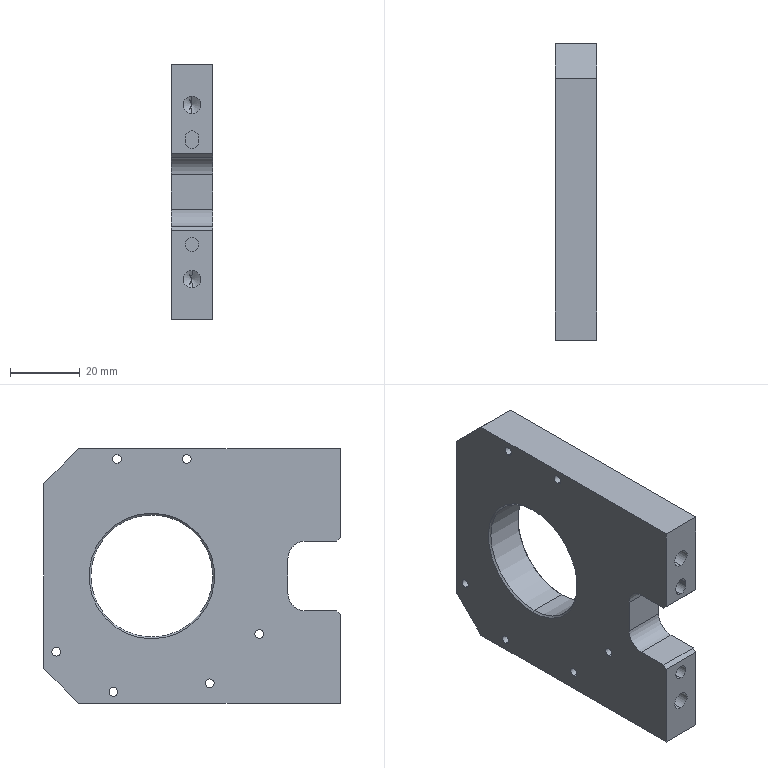Part | SolidWorks | features Chamfer 3, HoleWzd 2, Extrusion 1, ICE 1 | 1 solid | 51 faces | box 12 x 85 x 73 mm | volume 56726 mm3 | cylinder 25 | plane 18 | cone 8 | commonest cylinder face diameters 2.5 x12 4 x5 5 x4 10 x2 35 x2
STEP:
#1=CARTESIAN_POINT('',(5.5,54.,17.5));
#2=VERTEX_POINT('',#1);
#3=CARTESIAN_POINT('',(5.5,54.,-17.5));
#4=VERTEX_POINT('',#3);
#5=CARTESIAN_POINT('',(5.5,54.,0.));
#6=DIRECTION('',(1.,0.,0.));
#7=DIRECTION('',(0.,0.,1.));
#8=AXIS2_PLACEMENT_3D('',#5,#6,#7);
#9=CIRCLE('',#8,17.5);
#10=EDGE_CURVE('',#2,#4,#9,.T.);
#11=ORIENTED_EDGE('',*,*,#10,.F.);
#12=CARTESIAN_POINT('',(6.,54.,18.));
#13=VERTEX_POINT('',#12);
#14=CARTESIAN_POINT('',(5.5,54.,17.5));
#15=DIRECTION('',(0.7071,0.,0.7071));
#16=VECTOR('',#15,1000.);
#17=LINE('',#14,#16);
#18=EDGE_CURVE('',#2,#13,#17,.T.);
#19=ORIENTED_EDGE('',*,*,#18,.T.);
#20=CARTESIAN_POINT('',(6.,54.,-18.));
#21=VERTEX_POINT('',#20);
#22=CARTESIAN_POINT('',(6.,54.,0.));
#23=DIRECTION('',(-1.,0.,0.));
#24=DIRECTION('',(0.,0.,1.));
#25=AXIS2_PLACEMENT_3D('',#22,#23,#24);
#26=CIRCLE('',#25,18.);
#27=EDGE_CURVE('',#21,#13,#26,.T.);
#28=ORIENTED_EDGE('',*,*,#27,.F.);
#29=CARTESIAN_POINT('',(5.5,54.,-17.5));
#30=DIRECTION('',(0.7071,0.,-0.7071));
#31=VECTOR('',#30,1000.);
#32=LINE('',#29,#31);
#33=EDGE_CURVE('',#4,#21,#32,.T.);
#34=ORIENTED_EDGE('',*,*,#33,.F.);
#35=EDGE_LOOP('',(#11,#19,#28,#34));
#36=FACE_OUTER_BOUND('',#35,.T.);
#37=CARTESIAN_POINT('',(5.5,54.,0.));
#38=DIRECTION('',(1.,0.,0.));
#39=DIRECTION('',(0.,0.,-1.));
#40=AXIS2_PLACEMENT_3D('',#37,#38,#39);
#41=CONICAL_SURFACE('',#40,17.5,0.7854);
#42=ADVANCED_FACE('',(#36),#41,.F.);
#43=CARTESIAN_POINT('',(-5.5,54.,-17.5));
#44=VERTEX_POINT('',#43);
#45=CARTESIAN_POINT('',(-5.5,54.,17.5));
#46=VERTEX_POINT('',#45);
#47=CARTESIAN_POINT('',(-5.5,54.,0.));
#48=DIRECTION('',(-1.,0.,0.));
#49=DIRECTION('',(0.,0.,1.));
#50=AXIS2_PLACEMENT_3D('',#47,#48,#49);
#51=CIRCLE('',#50,17.5);
#52=EDGE_CURVE('',#44,#46,#51,.T.);
#53=ORIENTED_EDGE('',*,*,#52,.F.);
#54=CARTESIAN_POINT('',(-6.,54.,-18.));
#55=VERTEX_POINT('',#54);
#56=CARTESIAN_POINT('',(-6.,54.,-18.));
#57=DIRECTION('',(-0.7071,0.,-0.7071));
#58=VECTOR('',#57,1000.);
#59=LINE('',#56,#58);
#60=EDGE_CURVE('',#44,#55,#59,.T.);
#61=ORIENTED_EDGE('',*,*,#60,.T.);
#62=CARTESIAN_POINT('',(-6.,54.,18.));
#63=VERTEX_POINT('',#62);
#64=CARTESIAN_POINT('',(-6.,54.,0.));
#65=DIRECTION('',(1.,0.,0.));
#66=DIRECTION('',(0.,0.,1.));
#67=AXIS2_PLACEMENT_3D('',#64,#65,#66);
#68=CIRCLE('',#67,18.);
#69=EDGE_CURVE('',#63,#55,#68,.T.);
#70=ORIENTED_EDGE('',*,*,#69,.F.);
#71=CARTESIAN_POINT('',(-6.,54.,18.));
#72=DIRECTION('',(-0.7071,0.,0.7071));
#73=VECTOR('',#72,1000.);
#74=LINE('',#71,#73);
#75=EDGE_CURVE('',#46,#63,#74,.T.);
#76=ORIENTED_EDGE('',*,*,#75,.F.);
#77=EDGE_LOOP('',(#53,#61,#70,#76));
#78=FACE_OUTER_BOUND('',#77,.T.);
#79=CARTESIAN_POINT('',(-6.,54.,0.));
#80=DIRECTION('',(-1.,0.,0.));
#81=DIRECTION('',(0.,0.,1.));
#82=AXIS2_PLACEMENT_3D('',#79,#80,#81);
#83=CONICAL_SURFACE('',#82,18.,0.7854);
#84=ADVANCED_FACE('',(#78),#83,.F.);
#85=CARTESIAN_POINT('',(6.,44.,32.25));
#86=VERTEX_POINT('',#85);
#87=CARTESIAN_POINT('',(6.,44.,34.75));
#88=VERTEX_POINT('',#87);
#89=CARTESIAN_POINT('',(6.,44.,33.5));
#90=DIRECTION('',(-1.,0.,0.));
#91=DIRECTION('',(0.,0.,1.));
#92=AXIS2_PLACEMENT_3D('',#89,#90,#91);
#93=CIRCLE('',#92,1.25);
#94=EDGE_CURVE('',#86,#88,#93,.T.);
#95=ORIENTED_EDGE('',*,*,#94,.F.);
#96=CARTESIAN_POINT('',(-6.,44.,32.25));
#97=VERTEX_POINT('',#96);
#98=CARTESIAN_POINT('',(-6.,44.,32.25));
#99=DIRECTION('',(-1.,0.,0.));
#100=VECTOR('',#99,1000.);
#101=LINE('',#98,#100);
#102=EDGE_CURVE('',#86,#97,#101,.T.);
#103=ORIENTED_EDGE('',*,*,#102,.T.);
#104=CARTESIAN_POINT('',(-6.,44.,34.75));
#105=VERTEX_POINT('',#104);
#106=CARTESIAN_POINT('',(-6.,44.,33.5));
#107=DIRECTION('',(-1.,0.,0.));
#108=DIRECTION('',(0.,0.,1.));
#109=AXIS2_PLACEMENT_3D('',#106,#107,#108);
#110=CIRCLE('',#109,1.25);
#111=EDGE_CURVE('',#97,#105,#110,.T.);
#112=ORIENTED_EDGE('',*,*,#111,.T.);
#113=CARTESIAN_POINT('',(-6.,44.,34.75));
#114=DIRECTION('',(-1.,0.,0.));
#115=VECTOR('',#114,1000.);
#116=LINE('',#113,#115);
#117=EDGE_CURVE('',#88,#105,#116,.T.);
#118=ORIENTED_EDGE('',*,*,#117,.F.);
#119=EDGE_LOOP('',(#95,#103,#112,#118));
#120=FACE_OUTER_BOUND('',#119,.T.);
#121=CARTESIAN_POINT('',(-6.,44.,33.5));
#122=DIRECTION('',(-1.,0.,0.));
#123=DIRECTION('',(0.,0.,1.));
#124=AXIS2_PLACEMENT_3D('',#121,#122,#123);
#125=CYLINDRICAL_SURFACE('',#124,1.25);
#126=ADVANCED_FACE('',(#120),#125,.F.);
#127=CARTESIAN_POINT('',(6.,64.,32.25));
#128=VERTEX_POINT('',#127);
#129=CARTESIAN_POINT('',(6.,64.,34.75));
#130=VERTEX_POINT('',#129);
#131=CARTESIAN_POINT('',(6.,64.,33.5));
#132=DIRECTION('',(-1.,0.,0.));
#133=DIRECTION('',(0.,0.,1.));
#134=AXIS2_PLACEMENT_3D('',#131,#132,#133);
#135=CIRCLE('',#134,1.25);
#136=EDGE_CURVE('',#128,#130,#135,.T.);
#137=ORIENTED_EDGE('',*,*,#136,.F.);
#138=CARTESIAN_POINT('',(-6.,64.,32.25));
#139=VERTEX_POINT('',#138);
#140=CARTESIAN_POINT('',(-6.,64.,32.25));
#141=DIRECTION('',(-1.,0.,0.));
#142=VECTOR('',#141,1000.);
#143=LINE('',#140,#142);
#144=EDGE_CURVE('',#128,#139,#143,.T.);
#145=ORIENTED_EDGE('',*,*,#144,.T.);
#146=CARTESIAN_POINT('',(-6.,64.,34.75));
#147=VERTEX_POINT('',#146);
#148=CARTESIAN_POINT('',(-6.,64.,33.5));
#149=DIRECTION('',(-1.,0.,0.));
#150=DIRECTION('',(0.,0.,1.));
#151=AXIS2_PLACEMENT_3D('',#148,#149,#150);
#152=CIRCLE('',#151,1.25);
#153=EDGE_CURVE('',#139,#147,#152,.T.);
#154=ORIENTED_EDGE('',*,*,#153,.T.);
#155=CARTESIAN_POINT('',(-6.,64.,34.75));
#156=DIRECTION('',(-1.,0.,0.));
#157=VECTOR('',#156,1000.);
#158=LINE('',#155,#157);
#159=EDGE_CURVE('',#130,#147,#158,.T.);
#160=ORIENTED_EDGE('',*,*,#159,.F.);
#161=EDGE_LOOP('',(#137,#145,#154,#160));
#162=FACE_OUTER_BOUND('',#161,.T.);
#163=CARTESIAN_POINT('',(-6.,64.,33.5));
#164=DIRECTION('',(-1.,0.,0.));
#165=DIRECTION('',(0.,0.,1.));
#166=AXIS2_PLACEMENT_3D('',#163,#164,#165);
#167=CYLINDRICAL_SURFACE('',#166,1.25);
#168=ADVANCED_FACE('',(#162),#167,.F.);
#169=CARTESIAN_POINT('',(6.,23.241,-17.867));
#170=VERTEX_POINT('',#169);
#171=CARTESIAN_POINT('',(6.,23.241,-15.367));
#172=VERTEX_POINT('',#171);
#173=CARTESIAN_POINT('',(6.,23.241,-16.617));
#174=DIRECTION('',(-1.,0.,0.));
#175=DIRECTION('',(0.,0.,1.));
#176=AXIS2_PLACEMENT_3D('',#173,#174,#175);
#177=CIRCLE('',#176,1.25);
#178=EDGE_CURVE('',#170,#172,#177,.T.);
#179=ORIENTED_EDGE('',*,*,#178,.F.);
#180=CARTESIAN_POINT('',(-6.,23.241,-17.867));
#181=VERTEX_POINT('',#180);
#182=CARTESIAN_POINT('',(-6.,23.241,-17.867));
#183=DIRECTION('',(-1.,0.,0.));
#184=VECTOR('',#183,1000.);
#185=LINE('',#182,#184);
#186=EDGE_CURVE('',#170,#181,#185,.T.);
#187=ORIENTED_EDGE('',*,*,#186,.T.);
#188=CARTESIAN_POINT('',(-6.,23.241,-15.367));
#189=VERTEX_POINT('',#188);
#190=CARTESIAN_POINT('',(-6.,23.241,-16.617));
#191=DIRECTION('',(-1.,0.,0.));
#192=DIRECTION('',(0.,0.,1.));
#193=AXIS2_PLACEMENT_3D('',#190,#191,#192);
#194=CIRCLE('',#193,1.25);
#195=EDGE_CURVE('',#181,#189,#194,.T.);
#196=ORIENTED_EDGE('',*,*,#195,.T.);
#197=CARTESIAN_POINT('',(-6.,23.241,-15.367));
#198=DIRECTION('',(-1.,0.,0.));
#199=VECTOR('',#198,1000.);
#200=LINE('',#197,#199);
#201=EDGE_CURVE('',#172,#189,#200,.T.);
#202=ORIENTED_EDGE('',*,*,#201,.F.);
#203=EDGE_LOOP('',(#179,#187,#196,#202));
#204=FACE_OUTER_BOUND('',#203,.T.);
#205=CARTESIAN_POINT('',(-6.,23.241,-16.617));
#206=DIRECTION('',(-1.,0.,0.));
#207=DIRECTION('',(0.,0.,1.));
#208=AXIS2_PLACEMENT_3D('',#205,#206,#207);
#209=CYLINDRICAL_SURFACE('',#208,1.25);
#210=ADVANCED_FACE('',(#204),#209,.F.);
#211=CARTESIAN_POINT('',(6.,37.383,-32.009));
#212=VERTEX_POINT('',#211);
#213=CARTESIAN_POINT('',(6.,37.383,-29.509));
#214=VERTEX_POINT('',#213);
#215=CARTESIAN_POINT('',(6.,37.383,-30.759));
#216=DIRECTION('',(-1.,0.,0.));
#217=DIRECTION('',(0.,0.,1.));
#218=AXIS2_PLACEMENT_3D('',#215,#216,#217);
#219=CIRCLE('',#218,1.25);
#220=EDGE_CURVE('',#212,#214,#219,.T.);
#221=ORIENTED_EDGE('',*,*,#220,.F.);
#222=CARTESIAN_POINT('',(-6.,37.383,-32.009));
#223=VERTEX_POINT('',#222);
#224=CARTESIAN_POINT('',(-6.,37.383,-32.009));
#225=DIRECTION('',(-1.,0.,0.));
#226=VECTOR('',#225,1000.);
#227=LINE('',#224,#226);
#228=EDGE_CURVE('',#212,#223,#227,.T.);
#229=ORIENTED_EDGE('',*,*,#228,.T.);
#230=CARTESIAN_POINT('',(-6.,37.383,-29.509));
#231=VERTEX_POINT('',#230);
#232=CARTESIAN_POINT('',(-6.,37.383,-30.759));
#233=DIRECTION('',(-1.,0.,0.));
#234=DIRECTION('',(0.,0.,1.));
#235=AXIS2_PLACEMENT_3D('',#232,#233,#234);
#236=CIRCLE('',#235,1.25);
#237=EDGE_CURVE('',#223,#231,#236,.T.);
#238=ORIENTED_EDGE('',*,*,#237,.T.);
#239=CARTESIAN_POINT('',(-6.,37.383,-29.509));
#240=DIRECTION('',(-1.,0.,0.));
#241=VECTOR('',#240,1000.);
#242=LINE('',#239,#241);
#243=EDGE_CURVE('',#214,#231,#242,.T.);
#244=ORIENTED_EDGE('',*,*,#243,.F.);
#245=EDGE_LOOP('',(#221,#229,#238,#244));
#246=FACE_OUTER_BOUND('',#245,.T.);
#247=CARTESIAN_POINT('',(-6.,37.383,-30.759));
#248=DIRECTION('',(-1.,0.,0.));
#249=DIRECTION('',(0.,0.,1.));
#250=AXIS2_PLACEMENT_3D('',#247,#248,#249);
#251=CYLINDRICAL_SURFACE('',#250,1.25);
#252=ADVANCED_FACE('',(#246),#251,.F.);
#253=CARTESIAN_POINT('',(6.,65.023,-34.427));
#254=VERTEX_POINT('',#253);
#255=CARTESIAN_POINT('',(6.,65.023,-31.927));
#256=VERTEX_POINT('',#255);
#257=CARTESIAN_POINT('',(6.,65.023,-33.177));
#258=DIRECTION('',(-1.,0.,0.));
#259=DIRECTION('',(0.,0.,1.));
#260=AXIS2_PLACEMENT_3D('',#257,#258,#259);
#261=CIRCLE('',#260,1.25);
#262=EDGE_CURVE('',#254,#256,#261,.T.);
#263=ORIENTED_EDGE('',*,*,#262,.F.);
#264=CARTESIAN_POINT('',(-6.,65.023,-34.427));
#265=VERTEX_POINT('',#264);
#266=CARTESIAN_POINT('',(-6.,65.023,-34.427));
#267=DIRECTION('',(-1.,0.,0.));
#268=VECTOR('',#267,1000.);
#269=LINE('',#266,#268);
#270=EDGE_CURVE('',#254,#265,#269,.T.);
#271=ORIENTED_EDGE('',*,*,#270,.T.);
#272=CARTESIAN_POINT('',(-6.,65.023,-31.927));
#273=VERTEX_POINT('',#272);
#274=CARTESIAN_POINT('',(-6.,65.023,-33.177));
#275=DIRECTION('',(-1.,0.,0.));
#276=DIRECTION('',(0.,0.,1.));
#277=AXIS2_PLACEMENT_3D('',#274,#275,#276);
#278=CIRCLE('',#277,1.25);
#279=EDGE_CURVE('',#265,#273,#278,.T.);
#280=ORIENTED_EDGE('',*,*,#279,.T.);
#281=CARTESIAN_POINT('',(-6.,65.023,-31.927));
#282=DIRECTION('',(-1.,0.,0.));
#283=VECTOR('',#282,1000.);
#284=LINE('',#281,#283);
#285=EDGE_CURVE('',#256,#273,#284,.T.);
#286=ORIENTED_EDGE('',*,*,#285,.F.);
#287=EDGE_LOOP('',(#263,#271,#280,#286));
#288=FACE_OUTER_BOUND('',#287,.T.);
#289=CARTESIAN_POINT('',(-6.,65.023,-33.177));
#290=DIRECTION('',(-1.,0.,0.));
#291=DIRECTION('',(0.,0.,1.));
#292=AXIS2_PLACEMENT_3D('',#289,#290,#291);
#293=CYLINDRICAL_SURFACE('',#292,1.25);
#294=ADVANCED_FACE('',(#288),#293,.F.);
#295=CARTESIAN_POINT('',(6.,81.406,-22.956));
#296=VERTEX_POINT('',#295);
#297=CARTESIAN_POINT('',(6.,81.406,-20.456));
#298=VERTEX_POINT('',#297);
#299=CARTESIAN_POINT('',(6.,81.406,-21.706));
#300=DIRECTION('',(-1.,0.,0.));
#301=DIRECTION('',(0.,0.,1.));
#302=AXIS2_PLACEMENT_3D('',#299,#300,#301);
#303=CIRCLE('',#302,1.25);
#304=EDGE_CURVE('',#296,#298,#303,.T.);
#305=ORIENTED_EDGE('',*,*,#304,.F.);
#306=CARTESIAN_POINT('',(-6.,81.406,-22.956));
#307=VERTEX_POINT('',#306);
#308=CARTESIAN_POINT('',(-6.,81.406,-22.956));
#309=DIRECTION('',(-1.,0.,0.));
#310=VECTOR('',#309,1000.);
#311=LINE('',#308,#310);
#312=EDGE_CURVE('',#296,#307,#311,.T.);
#313=ORIENTED_EDGE('',*,*,#312,.T.);
#314=CARTESIAN_POINT('',(-6.,81.406,-20.456));
#315=VERTEX_POINT('',#314);
#316=CARTESIAN_POINT('',(-6.,81.406,-21.706));
#317=DIRECTION('',(-1.,0.,0.));
#318=DIRECTION('',(0.,0.,1.));
#319=AXIS2_PLACEMENT_3D('',#316,#317,#318);
#320=CIRCLE('',#319,1.25);
#321=EDGE_CURVE('',#307,#315,#320,.T.);
#322=ORIENTED_EDGE('',*,*,#321,.T.);
#323=CARTESIAN_POINT('',(-6.,81.406,-20.456));
#324=DIRECTION('',(-1.,0.,0.));
#325=VECTOR('',#324,1000.);
#326=LINE('',#323,#325);
#327=EDGE_CURVE('',#298,#315,#326,.T.);
#328=ORIENTED_EDGE('',*,*,#327,.F.);
#329=EDGE_LOOP('',(#305,#313,#322,#328));
#330=FACE_OUTER_BOUND('',#329,.T.);
#331=CARTESIAN_POINT('',(-6.,81.406,-21.706));
#332=DIRECTION('',(-1.,0.,0.));
#333=DIRECTION('',(0.,0.,1.));
#334=AXIS2_PLACEMENT_3D('',#331,#332,#333);
#335=CYLINDRICAL_SURFACE('',#334,1.25);
#336=ADVANCED_FACE('',(#330),#335,.F.);
#337=CARTESIAN_POINT('',(0.,15.,12.5));
#338=VERTEX_POINT('',#337);
#339=CARTESIAN_POINT('',(2.,15.,14.5));
#340=VERTEX_POINT('',#339);
#341=CARTESIAN_POINT('',(0.,15.,14.5));
#342=DIRECTION('',(0.,-1.,0.));
#343=DIRECTION('',(0.,0.,-1.));
#344=AXIS2_PLACEMENT_3D('',#341,#342,#343);
#345=CIRCLE('',#344,2.);
#346=EDGE_CURVE('',#338,#340,#345,.T.);
#347=ORIENTED_EDGE('',*,*,#346,.F.);
#348=CARTESIAN_POINT('',(0.,0.,12.5));
#349=VERTEX_POINT('',#348);
#350=CARTESIAN_POINT('',(0.,15.,12.5));
#351=DIRECTION('',(0.,-1.,0.));
#352=VECTOR('',#351,1000.);
#353=LINE('',#350,#352);
#354=EDGE_CURVE('',#338,#349,#353,.T.);
#355=ORIENTED_EDGE('',*,*,#354,.T.);
#356=CARTESIAN_POINT('',(2.,0.,14.5));
#357=VERTEX_POINT('',#356);
#358=CARTESIAN_POINT('',(0.,0.,14.5));
#359=DIRECTION('',(0.,-1.,0.));
#360=DIRECTION('',(0.,0.,-1.));
#361=AXIS2_PLACEMENT_3D('',#358,#359,#360);
#362=CIRCLE('',#361,2.);
#363=EDGE_CURVE('',#349,#357,#362,.T.);
#364=ORIENTED_EDGE('',*,*,#363,.T.);
#365=CARTESIAN_POINT('',(2.,15.,14.5));
#366=DIRECTION('',(0.,-1.,0.));
#367=VECTOR('',#366,1000.);
#368=LINE('',#365,#367);
#369=EDGE_CURVE('',#340,#357,#368,.T.);
#370=ORIENTED_EDGE('',*,*,#369,.F.);
#371=EDGE_LOOP('',(#347,#355,#364,#370));
#372=FACE_OUTER_BOUND('',#371,.T.);
#373=CARTESIAN_POINT('',(0.,15.,14.5));
#374=DIRECTION('',(0.,-1.,0.));
#375=DIRECTION('',(0.,0.,-1.));
#376=AXIS2_PLACEMENT_3D('',#373,#374,#375);
#377=CYLINDRICAL_SURFACE('',#376,2.);
#378=ADVANCED_FACE('',(#372),#377,.F.);
#379=CARTESIAN_POINT('',(0.,15.,-13.));
#380=VERTEX_POINT('',#379);
#381=CARTESIAN_POINT('',(0.,15.,-17.));
#382=VERTEX_POINT('',#381);
#383=CARTESIAN_POINT('',(0.,15.,-15.));
#384=DIRECTION('',(0.,-1.,0.));
#385=DIRECTION('',(0.,0.,-1.));
#386=AXIS2_PLACEMENT_3D('',#383,#384,#385);
#387=CIRCLE('',#386,2.);
#388=EDGE_CURVE('',#380,#382,#387,.T.);
#389=ORIENTED_EDGE('',*,*,#388,.F.);
#390=CARTESIAN_POINT('',(0.,0.,-13.));
#391=VERTEX_POINT('',#390);
#392=CARTESIAN_POINT('',(0.,15.,-13.));
#393=DIRECTION('',(0.,-1.,0.));
#394=VECTOR('',#393,1000.);
#395=LINE('',#392,#394);
#396=EDGE_CURVE('',#380,#391,#395,.T.);
#397=ORIENTED_EDGE('',*,*,#396,.T.);
#398=CARTESIAN_POINT('',(0.,0.,-17.));
#399=VERTEX_POINT('',#398);
#400=CARTESIAN_POINT('',(0.,0.,-15.));
#401=DIRECTION('',(0.,-1.,0.));
#402=DIRECTION('',(0.,0.,-1.));
#403=AXIS2_PLACEMENT_3D('',#400,#401,#402);
#404=CIRCLE('',#403,2.);
#405=EDGE_CURVE('',#391,#399,#404,.T.);
#406=ORIENTED_EDGE('',*,*,#405,.T.);
#407=CARTESIAN_POINT('',(0.,15.,-17.));
#408=DIRECTION('',(0.,-1.,0.));
#409=VECTOR('',#408,1000.);
#410=LINE('',#407,#409);
#411=EDGE_CURVE('',#382,#399,#410,.T.);
#412=ORIENTED_EDGE('',*,*,#411,.F.);
#413=EDGE_LOOP('',(#389,#397,#406,#412));
#414=FACE_OUTER_BOUND('',#413,.T.);
#415=CARTESIAN_POINT('',(0.,15.,-15.));
#416=DIRECTION('',(0.,-1.,0.));
#417=DIRECTION('',(0.,0.,-1.));
#418=AXIS2_PLACEMENT_3D('',#415,#416,#417);
#419=CYLINDRICAL_SURFACE('',#418,2.);
#420=ADVANCED_FACE('',(#414),#419,.F.);
#421=CARTESIAN_POINT('',(0.,17.,27.5));
#422=VERTEX_POINT('',#421);
#423=CARTESIAN_POINT('',(0.,17.,22.5));
#424=VERTEX_POINT('',#423);
#425=CARTESIAN_POINT('',(0.,17.,25.));
#426=DIRECTION('',(0.,-1.,0.));
#427=DIRECTION('',(0.,0.,-1.));
#428=AXIS2_PLACEMENT_3D('',#425,#426,#427);
#429=CIRCLE('',#428,2.5);
#430=EDGE_CURVE('',#422,#424,#429,.T.);
#431=ORIENTED_EDGE('',*,*,#430,.F.);
#432=CARTESIAN_POINT('',(0.,0.,27.5));
#433=VERTEX_POINT('',#432);
#434=CARTESIAN_POINT('',(0.,0.,27.5));
#435=DIRECTION('',(0.,-1.,0.));
#436=VECTOR('',#435,1000.);
#437=LINE('',#434,#436);
#438=EDGE_CURVE('',#422,#433,#437,.T.);
#439=ORIENTED_EDGE('',*,*,#438,.T.);
#440=CARTESIAN_POINT('',(0.,0.,22.5));
#441=VERTEX_POINT('',#440);
#442=CARTESIAN_POINT('',(0.,0.,25.));
#443=DIRECTION('',(0.,-1.,0.));
#444=DIRECTION('',(0.,0.,-1.));
#445=AXIS2_PLACEMENT_3D('',#442,#443,#444);
#446=CIRCLE('',#445,2.5);
#447=EDGE_CURVE('',#433,#441,#446,.T.);
#448=ORIENTED_EDGE('',*,*,#447,.T.);
#449=CARTESIAN_POINT('',(0.,0.,22.5));
#450=DIRECTION('',(0.,-1.,0.));
#451=VECTOR('',#450,1000.);
#452=LINE('',#449,#451);
#453=EDGE_CURVE('',#424,#441,#452,.T.);
#454=ORIENTED_EDGE('',*,*,#453,.F.);
#455=EDGE_LOOP('',(#431,#439,#448,#454));
#456=FACE_OUTER_BOUND('',#455,.T.);
#457=CARTESIAN_POINT('',(0.,0.,25.));
#458=DIRECTION('',(0.,-1.,0.));
#459=DIRECTION('',(0.,0.,-1.));
#460=AXIS2_PLACEMENT_3D('',#457,#458,#459);
#461=CYLINDRICAL_SURFACE('',#460,2.5);
#462=ADVANCED_FACE('',(#456),#461,.F.);
#463=CARTESIAN_POINT('',(0.,18.502,25.));
#464=VERTEX_POINT('',#463);
#465=CARTESIAN_POINT('',(0.,17.,22.5));
#466=DIRECTION('',(0.,-0.515,-0.8572));
#467=VECTOR('',#466,1000.);
#468=LINE('',#465,#467);
#469=EDGE_CURVE('',#464,#424,#468,.T.);
#470=ORIENTED_EDGE('',*,*,#469,.F.);
#471=CARTESIAN_POINT('',(0.,17.,27.5));
#472=DIRECTION('',(0.,-0.515,0.8572));
#473=VECTOR('',#472,1000.);
#474=LINE('',#471,#473);
#475=EDGE_CURVE('',#464,#422,#474,.T.);
#476=ORIENTED_EDGE('',*,*,#475,.T.);
#477=ORIENTED_EDGE('',*,*,#430,.T.);
#478=EDGE_LOOP('',(#470,#476,#477));
#479=FACE_OUTER_BOUND('',#478,.T.);
#480=CARTESIAN_POINT('',(0.,17.,25.));
#481=DIRECTION('',(0.,-1.,0.));
#482=DIRECTION('',(0.,0.,-1.));
#483=AXIS2_PLACEMENT_3D('',#480,#481,#482);
#484=CONICAL_SURFACE('',#483,2.5,1.03);
#485=ADVANCED_FACE('',(#479),#484,.F.);
#486=CARTESIAN_POINT('',(0.,17.,-22.5));
#487=VERTEX_POINT('',#486);
#488=CARTESIAN_POINT('',(0.,17.,-27.5));
#489=VERTEX_POINT('',#488);
#490=CARTESIAN_POINT('',(0.,17.,-25.));
#491=DIRECTION('',(0.,-1.,0.));
#492=DIRECTION('',(0.,0.,-1.));
#493=AXIS2_PLACEMENT_3D('',#490,#491,#492);
#494=CIRCLE('',#493,2.5);
#495=EDGE_CURVE('',#487,#489,#494,.T.);
#496=ORIENTED_EDGE('',*,*,#495,.F.);
#497=CARTESIAN_POINT('',(0.,0.,-22.5));
#498=VERTEX_POINT('',#497);
#499=CARTESIAN_POINT('',(0.,0.,-22.5));
#500=DIRECTION('',(0.,-1.,0.));
#501=VECTOR('',#500,1000.);
#502=LINE('',#499,#501);
#503=EDGE_CURVE('',#487,#498,#502,.T.);
#504=ORIENTED_EDGE('',*,*,#503,.T.);
#505=CARTESIAN_POINT('',(0.,0.,-27.5));
#506=VERTEX_POINT('',#505);
#507=CARTESIAN_POINT('',(0.,0.,-25.));
#508=DIRECTION('',(0.,-1.,0.));
#509=DIRECTION('',(0.,0.,-1.));
#510=AXIS2_PLACEMENT_3D('',#507,#508,#509);
#511=CIRCLE('',#510,2.5);
#512=EDGE_CURVE('',#498,#506,#511,.T.);
#513=ORIENTED_EDGE('',*,*,#512,.T.);
#514=CARTESIAN_POINT('',(0.,0.,-27.5));
#515=DIRECTION('',(0.,-1.,0.));
#516=VECTOR('',#515,1000.);
#517=LINE('',#514,#516);
#518=EDGE_CURVE('',#489,#506,#517,.T.);
#519=ORIENTED_EDGE('',*,*,#518,.F.);
#520=EDGE_LOOP('',(#496,#504,#513,#519));
#521=FACE_OUTER_BOUND('',#520,.T.);
#522=CARTESIAN_POINT('',(0.,0.,-25.));
#523=DIRECTION('',(0.,-1.,0.));
#524=DIRECTION('',(0.,0.,-1.));
#525=AXIS2_PLACEMENT_3D('',#522,#523,#524);
#526=CYLINDRICAL_SURFACE('',#525,2.5);
#527=ADVANCED_FACE('',(#521),#526,.F.);
#528=CARTESIAN_POINT('',(0.,18.502,-25.));
#529=VERTEX_POINT('',#528);
#530=CARTESIAN_POINT('',(0.,17.,-27.5));
#531=DIRECTION('',(0.,-0.515,-0.8572));
#532=VECTOR('',#531,1000.);
#533=LINE('',#530,#532);
#534=EDGE_CURVE('',#529,#489,#533,.T.);
#535=ORIENTED_EDGE('',*,*,#534,.F.);
#536=CARTESIAN_POINT('',(0.,17.,-22.5));
#537=DIRECTION('',(0.,-0.515,0.8572));
#538=VECTOR('',#537,1000.);
#539=LINE('',#536,#538);
#540=EDGE_CURVE('',#529,#487,#539,.T.);
#541=ORIENTED_EDGE('',*,*,#540,.T.);
#542=ORIENTED_EDGE('',*,*,#495,.T.);
#543=EDGE_LOOP('',(#535,#541,#542));
#544=FACE_OUTER_BOUND('',#543,.T.);
#545=CARTESIAN_POINT('',(0.,17.,-25.));
#546=DIRECTION('',(0.,-1.,0.));
#547=DIRECTION('',(0.,0.,-1.));
#548=AXIS2_PLACEMENT_3D('',#545,#546,#547);
#549=CONICAL_SURFACE('',#548,2.5,1.03);
#550=ADVANCED_FACE('',(#544),#549,.F.);
#551=ORIENTED_EDGE('',*,*,#10,.T.);
#552=CARTESIAN_POINT('',(6.,54.,-17.5));
#553=DIRECTION('',(-1.,0.,0.));
#554=VECTOR('',#553,1000.);
#555=LINE('',#552,#554);
#556=EDGE_CURVE('',#4,#44,#555,.T.);
#557=ORIENTED_EDGE('',*,*,#556,.T.);
#558=ORIENTED_EDGE('',*,*,#52,.T.);
#559=CARTESIAN_POINT('',(6.,54.,17.5));
#560=DIRECTION('',(-1.,0.,0.));
#561=VECTOR('',#560,1000.);
#562=LINE('',#559,#561);
#563=EDGE_CURVE('',#2,#46,#562,.T.);
#564=ORIENTED_EDGE('',*,*,#563,.F.);
#565=EDGE_LOOP('',(#551,#557,#558,#564));
#566=FACE_OUTER_BOUND('',#565,.T.);
#567=CARTESIAN_POINT('',(6.,54.,0.));
#568=DIRECTION('',(-1.,0.,0.));
#569=DIRECTION('',(0.,0.,1.));
#570=AXIS2_PLACEMENT_3D('',#567,#568,#569);
#571=CYLINDRICAL_SURFACE('',#570,17.5);
#572=ADVANCED_FACE('',(#566),#571,.F.);
#573=ORIENTED_EDGE('',*,*,#27,.T.);
#574=CARTESIAN_POINT('',(6.,54.,0.));
#575=DIRECTION('',(-1.,0.,0.));
#576=DIRECTION('',(0.,0.,1.));
#577=AXIS2_PLACEMENT_3D('',#574,#575,#576);
#578=CIRCLE('',#577,18.);
#579=EDGE_CURVE('',#13,#21,#578,.T.);
#580=ORIENTED_EDGE('',*,*,#579,.T.);
#581=EDGE_LOOP('',(#573,#580));
#582=FACE_BOUND('',#581,.T.);
#583=CARTESIAN_POINT('',(6.,44.,33.5));
#584=DIRECTION('',(-1.,0.,0.));
#585=DIRECTION('',(0.,0.,1.));
#586=AXIS2_PLACEMENT_3D('',#583,#584,#585);
#587=CIRCLE('',#586,1.25);
#588=EDGE_CURVE('',#88,#86,#587,.T.);
#589=ORIENTED_EDGE('',*,*,#588,.T.);
#590=ORIENTED_EDGE('',*,*,#94,.T.);
#591=EDGE_LOOP('',(#589,#590));
#592=FACE_BOUND('',#591,.T.);
#593=CARTESIAN_POINT('',(6.,64.,33.5));
#594=DIRECTION('',(-1.,0.,0.));
#595=DIRECTION('',(0.,0.,1.));
#596=AXIS2_PLACEMENT_3D('',#593,#594,#595);
#597=CIRCLE('',#596,1.25);
#598=EDGE_CURVE('',#130,#128,#597,.T.);
#599=ORIENTED_EDGE('',*,*,#598,.T.);
#600=ORIENTED_EDGE('',*,*,#136,.T.);
#601=EDGE_LOOP('',(#599,#600));
#602=FACE_BOUND('',#601,.T.);
#603=CARTESIAN_POINT('',(6.,23.241,-16.617));
#604=DIRECTION('',(-1.,0.,0.));
#605=DIRECTION('',(0.,0.,1.));
#606=AXIS2_PLACEMENT_3D('',#603,#604,#605);
#607=CIRCLE('',#606,1.25);
#608=EDGE_CURVE('',#172,#170,#607,.T.);
#609=ORIENTED_EDGE('',*,*,#608,.T.);
#610=ORIENTED_EDGE('',*,*,#178,.T.);
#611=EDGE_LOOP('',(#609,#610));
#612=FACE_BOUND('',#611,.T.);
#613=CARTESIAN_POINT('',(6.,37.383,-30.759));
#614=DIRECTION('',(-1.,0.,0.));
#615=DIRECTION('',(0.,0.,1.));
#616=AXIS2_PLACEMENT_3D('',#613,#614,#615);
#617=CIRCLE('',#616,1.25);
#618=EDGE_CURVE('',#214,#212,#617,.T.);
#619=ORIENTED_EDGE('',*,*,#618,.T.);
#620=ORIENTED_EDGE('',*,*,#220,.T.);
#621=EDGE_LOOP('',(#619,#620));
#622=FACE_BOUND('',#621,.T.);
#623=CARTESIAN_POINT('',(6.,65.023,-33.177));
#624=DIRECTION('',(-1.,0.,0.));
#625=DIRECTION('',(0.,0.,1.));
#626=AXIS2_PLACEMENT_3D('',#623,#624,#625);
#627=CIRCLE('',#626,1.25);
#628=EDGE_CURVE('',#256,#254,#627,.T.);
#629=ORIENTED_EDGE('',*,*,#628,.T.);
#630=ORIENTED_EDGE('',*,*,#262,.T.);
#631=EDGE_LOOP('',(#629,#630));
#632=FACE_BOUND('',#631,.T.);
#633=CARTESIAN_POINT('',(6.,81.406,-21.706));
#634=DIRECTION('',(-1.,0.,0.));
#635=DIRECTION('',(0.,0.,1.));
#636=AXIS2_PLACEMENT_3D('',#633,#634,#635);
#637=CIRCLE('',#636,1.25);
#638=EDGE_CURVE('',#298,#296,#637,.T.);
#639=ORIENTED_EDGE('',*,*,#638,.T.);
#640=ORIENTED_EDGE('',*,*,#304,.T.);
#641=EDGE_LOOP('',(#639,#640));
#642=FACE_BOUND('',#641,.T.);
#643=CARTESIAN_POINT('',(6.,0.,36.5));
#644=VERTEX_POINT('',#643);
#645=CARTESIAN_POINT('',(6.,0.,11.));
#646=VERTEX_POINT('',#645);
#647=CARTESIAN_POINT('',(6.,0.,36.5));
#648=DIRECTION('',(0.,0.,-1.));
#649=VECTOR('',#648,1000.);
#650=LINE('',#647,#649);
#651=EDGE_CURVE('',#644,#646,#650,.T.);
#652=ORIENTED_EDGE('',*,*,#651,.T.);
#653=CARTESIAN_POINT('',(6.,1.,10.));
#654=VERTEX_POINT('',#653);
#655=CARTESIAN_POINT('',(6.,1.,10.));
#656=DIRECTION('',(0.,0.7071,-0.7071));
#657=VECTOR('',#656,1000.);
#658=LINE('',#655,#657);
#659=EDGE_CURVE('',#646,#654,#658,.T.);
#660=ORIENTED_EDGE('',*,*,#659,.T.);
#661=CARTESIAN_POINT('',(6.,10.,10.));
#662=VERTEX_POINT('',#661);
#663=CARTESIAN_POINT('',(6.,0.,10.));
#664=DIRECTION('',(0.,1.,0.));
#665=VECTOR('',#664,1000.);
#666=LINE('',#663,#665);
#667=EDGE_CURVE('',#654,#662,#666,.T.);
#668=ORIENTED_EDGE('',*,*,#667,.T.);
#669=CARTESIAN_POINT('',(6.,15.,5.));
#670=VERTEX_POINT('',#669);
#671=CARTESIAN_POINT('',(6.,10.,5.));
#672=DIRECTION('',(-1.,0.,0.));
#673=DIRECTION('',(0.,0.,1.));
#674=AXIS2_PLACEMENT_3D('',#671,#672,#673);
#675=CIRCLE('',#674,5.);
#676=EDGE_CURVE('',#662,#670,#675,.T.);
#677=ORIENTED_EDGE('',*,*,#676,.T.);
#678=CARTESIAN_POINT('',(6.,15.,-5.));
#679=VERTEX_POINT('',#678);
#680=CARTESIAN_POINT('',(6.,15.,5.));
#681=DIRECTION('',(0.,0.,-1.));
#682=VECTOR('',#681,1000.);
#683=LINE('',#680,#682);
#684=EDGE_CURVE('',#670,#679,#683,.T.);
#685=ORIENTED_EDGE('',*,*,#684,.T.);
#686=CARTESIAN_POINT('',(6.,10.,-10.));
#687=VERTEX_POINT('',#686);
#688=CARTESIAN_POINT('',(6.,10.,-5.));
#689=DIRECTION('',(-1.,0.,0.));
#690=DIRECTION('',(0.,0.,1.));
#691=AXIS2_PLACEMENT_3D('',#688,#689,#690);
#692=CIRCLE('',#691,5.);
#693=EDGE_CURVE('',#679,#687,#692,.T.);
#694=ORIENTED_EDGE('',*,*,#693,.T.);
#695=CARTESIAN_POINT('',(6.,1.,-10.));
#696=VERTEX_POINT('',#695);
#697=CARTESIAN_POINT('',(6.,0.,-10.));
#698=DIRECTION('',(0.,-1.,0.));
#699=VECTOR('',#698,1000.);
#700=LINE('',#697,#699);
#701=EDGE_CURVE('',#687,#696,#700,.T.);
#702=ORIENTED_EDGE('',*,*,#701,.T.);
#703=CARTESIAN_POINT('',(6.,0.,-11.));
#704=VERTEX_POINT('',#703);
#705=CARTESIAN_POINT('',(6.,0.,-11.));
#706=DIRECTION('',(0.,-0.7071,-0.7071));
#707=VECTOR('',#706,1000.);
#708=LINE('',#705,#707);
#709=EDGE_CURVE('',#696,#704,#708,.T.);
#710=ORIENTED_EDGE('',*,*,#709,.T.);
#711=CARTESIAN_POINT('',(6.,0.,-36.5));
#712=VERTEX_POINT('',#711);
#713=CARTESIAN_POINT('',(6.,0.,-10.));
#714=DIRECTION('',(0.,0.,-1.));
#715=VECTOR('',#714,1000.);
#716=LINE('',#713,#715);
#717=EDGE_CURVE('',#704,#712,#716,.T.);
#718=ORIENTED_EDGE('',*,*,#717,.T.);
#719=CARTESIAN_POINT('',(6.,75.,-36.5));
#720=VERTEX_POINT('',#719);
#721=CARTESIAN_POINT('',(6.,0.,-36.5));
#722=DIRECTION('',(0.,1.,0.));
#723=VECTOR('',#722,1000.);
#724=LINE('',#721,#723);
#725=EDGE_CURVE('',#712,#720,#724,.T.);
#726=ORIENTED_EDGE('',*,*,#725,.T.);
#727=CARTESIAN_POINT('',(6.,85.,-26.5));
#728=VERTEX_POINT('',#727);
#729=CARTESIAN_POINT('',(6.,85.,-26.5));
#730=DIRECTION('',(0.,0.7071,0.7071));
#731=VECTOR('',#730,1000.);
#732=LINE('',#729,#731);
#733=EDGE_CURVE('',#720,#728,#732,.T.);
#734=ORIENTED_EDGE('',*,*,#733,.T.);
#735=CARTESIAN_POINT('',(6.,85.,26.5));
#736=VERTEX_POINT('',#735);
#737=CARTESIAN_POINT('',(6.,85.,36.5));
#738=DIRECTION('',(0.,0.,1.));
#739=VECTOR('',#738,1000.);
#740=LINE('',#737,#739);
#741=EDGE_CURVE('',#728,#736,#740,.T.);
#742=ORIENTED_EDGE('',*,*,#741,.T.);
#743=CARTESIAN_POINT('',(6.,75.,36.5));
#744=VERTEX_POINT('',#743);
#745=CARTESIAN_POINT('',(6.,75.,36.5));
#746=DIRECTION('',(0.,-0.7071,0.7071));
#747=VECTOR('',#746,1000.);
#748=LINE('',#745,#747);
#749=EDGE_CURVE('',#736,#744,#748,.T.);
#750=ORIENTED_EDGE('',*,*,#749,.T.);
#751=CARTESIAN_POINT('',(6.,0.,36.5));
#752=DIRECTION('',(0.,-1.,0.));
#753=VECTOR('',#752,1000.);
#754=LINE('',#751,#753);
#755=EDGE_CURVE('',#744,#644,#754,.T.);
#756=ORIENTED_EDGE('',*,*,#755,.T.);
#757=EDGE_LOOP('',(#652,#660,#668,#677,#685,#694,#702,#710,#718,#726,#734,#742,#750,#756));
#758=FACE_OUTER_BOUND('',#757,.T.);
#759=CARTESIAN_POINT('',(6.,10.,-5.));
#760=DIRECTION('',(-1.,0.,0.));
#761=DIRECTION('',(0.,0.,1.));
#762=AXIS2_PLACEMENT_3D('',#759,#760,#761);
#763=PLANE('',#762);
#764=ADVANCED_FACE('',(#582,#592,#602,#612,#622,#632,#642,#758),#763,.F.);
#765=ORIENTED_EDGE('',*,*,#69,.T.);
#766=CARTESIAN_POINT('',(-6.,54.,0.));
#767=DIRECTION('',(1.,0.,0.));
#768=DIRECTION('',(0.,0.,1.));
#769=AXIS2_PLACEMENT_3D('',#766,#767,#768);
#770=CIRCLE('',#769,18.);
#771=EDGE_CURVE('',#55,#63,#770,.T.);
#772=ORIENTED_EDGE('',*,*,#771,.T.);
#773=EDGE_LOOP('',(#765,#772));
#774=FACE_BOUND('',#773,.T.);
#775=CARTESIAN_POINT('',(-6.,44.,33.5));
#776=DIRECTION('',(-1.,0.,0.));
#777=DIRECTION('',(0.,0.,1.));
#778=AXIS2_PLACEMENT_3D('',#775,#776,#777);
#779=CIRCLE('',#778,1.25);
#780=EDGE_CURVE('',#105,#97,#779,.T.);
#781=ORIENTED_EDGE('',*,*,#780,.F.);
#782=ORIENTED_EDGE('',*,*,#111,.F.);
#783=EDGE_LOOP('',(#781,#782));
#784=FACE_BOUND('',#783,.T.);
#785=CARTESIAN_POINT('',(-6.,64.,33.5));
#786=DIRECTION('',(-1.,0.,0.));
#787=DIRECTION('',(0.,0.,1.));
#788=AXIS2_PLACEMENT_3D('',#785,#786,#787);
#789=CIRCLE('',#788,1.25);
#790=EDGE_CURVE('',#147,#139,#789,.T.);
#791=ORIENTED_EDGE('',*,*,#790,.F.);
#792=ORIENTED_EDGE('',*,*,#153,.F.);
#793=EDGE_LOOP('',(#791,#792));
#794=FACE_BOUND('',#793,.T.);
#795=CARTESIAN_POINT('',(-6.,23.241,-16.617));
#796=DIRECTION('',(-1.,0.,0.));
#797=DIRECTION('',(0.,0.,1.));
#798=AXIS2_PLACEMENT_3D('',#795,#796,#797);
#799=CIRCLE('',#798,1.25);
#800=EDGE_CURVE('',#189,#181,#799,.T.);
#801=ORIENTED_EDGE('',*,*,#800,.F.);
#802=ORIENTED_EDGE('',*,*,#195,.F.);
#803=EDGE_LOOP('',(#801,#802));
#804=FACE_BOUND('',#803,.T.);
#805=CARTESIAN_POINT('',(-6.,37.383,-30.759));
#806=DIRECTION('',(-1.,0.,0.));
#807=DIRECTION('',(0.,0.,1.));
#808=AXIS2_PLACEMENT_3D('',#805,#806,#807);
#809=CIRCLE('',#808,1.25);
#810=EDGE_CURVE('',#231,#223,#809,.T.);
#811=ORIENTED_EDGE('',*,*,#810,.F.);
#812=ORIENTED_EDGE('',*,*,#237,.F.);
#813=EDGE_LOOP('',(#811,#812));
#814=FACE_BOUND('',#813,.T.);
#815=CARTESIAN_POINT('',(-6.,65.023,-33.177));
#816=DIRECTION('',(-1.,0.,0.));
#817=DIRECTION('',(0.,0.,1.));
#818=AXIS2_PLACEMENT_3D('',#815,#816,#817);
#819=CIRCLE('',#818,1.25);
#820=EDGE_CURVE('',#273,#265,#819,.T.);
#821=ORIENTED_EDGE('',*,*,#820,.F.);
#822=ORIENTED_EDGE('',*,*,#279,.F.);
#823=EDGE_LOOP('',(#821,#822));
#824=FACE_BOUND('',#823,.T.);
#825=CARTESIAN_POINT('',(-6.,81.406,-21.706));
#826=DIRECTION('',(-1.,0.,0.));
#827=DIRECTION('',(0.,0.,1.));
#828=AXIS2_PLACEMENT_3D('',#825,#826,#827);
#829=CIRCLE('',#828,1.25);
#830=EDGE_CURVE('',#315,#307,#829,.T.);
#831=ORIENTED_EDGE('',*,*,#830,.F.);
#832=ORIENTED_EDGE('',*,*,#321,.F.);
#833=EDGE_LOOP('',(#831,#832));
#834=FACE_BOUND('',#833,.T.);
#835=CARTESIAN_POINT('',(-6.,1.,10.));
#836=VERTEX_POINT('',#835);
#837=CARTESIAN_POINT('',(-6.,10.,10.));
#838=VERTEX_POINT('',#837);
#839=CARTESIAN_POINT('',(-6.,0.,10.));
#840=DIRECTION('',(0.,1.,0.));
#841=VECTOR('',#840,1000.);
#842=LINE('',#839,#841);
#843=EDGE_CURVE('',#836,#838,#842,.T.);
#844=ORIENTED_EDGE('',*,*,#843,.F.);
#845=CARTESIAN_POINT('',(-6.,0.,11.));
#846=VERTEX_POINT('',#845);
#847=CARTESIAN_POINT('',(-6.,13.,-2.));
#848=DIRECTION('',(0.,-0.7071,0.7071));
#849=VECTOR('',#848,1000.);
#850=LINE('',#847,#849);
#851=EDGE_CURVE('',#836,#846,#850,.T.);
#852=ORIENTED_EDGE('',*,*,#851,.T.);
#853=CARTESIAN_POINT('',(-6.,0.,36.5));
#854=VERTEX_POINT('',#853);
#855=CARTESIAN_POINT('',(-6.,0.,36.5));
#856=DIRECTION('',(0.,0.,-1.));
#857=VECTOR('',#856,1000.);
#858=LINE('',#855,#857);
#859=EDGE_CURVE('',#854,#846,#858,.T.);
#860=ORIENTED_EDGE('',*,*,#859,.F.);
#861=CARTESIAN_POINT('',(-6.,75.,36.5));
#862=VERTEX_POINT('',#861);
#863=CARTESIAN_POINT('',(-6.,0.,36.5));
#864=DIRECTION('',(0.,-1.,0.));
#865=VECTOR('',#864,1000.);
#866=LINE('',#863,#865);
#867=EDGE_CURVE('',#862,#854,#866,.T.);
#868=ORIENTED_EDGE('',*,*,#867,.F.);
#869=CARTESIAN_POINT('',(-6.,85.,26.5));
#870=VERTEX_POINT('',#869);
#871=CARTESIAN_POINT('',(-6.,63.25,48.25));
#872=DIRECTION('',(0.,0.7071,-0.7071));
#873=VECTOR('',#872,1000.);
#874=LINE('',#871,#873);
#875=EDGE_CURVE('',#862,#870,#874,.T.);
#876=ORIENTED_EDGE('',*,*,#875,.T.);
#877=CARTESIAN_POINT('',(-6.,85.,-26.5));
#878=VERTEX_POINT('',#877);
#879=CARTESIAN_POINT('',(-6.,85.,36.5));
#880=DIRECTION('',(0.,0.,1.));
#881=VECTOR('',#880,1000.);
#882=LINE('',#879,#881);
#883=EDGE_CURVE('',#878,#870,#882,.T.);
#884=ORIENTED_EDGE('',*,*,#883,.F.);
#885=CARTESIAN_POINT('',(-6.,75.,-36.5));
#886=VERTEX_POINT('',#885);
#887=CARTESIAN_POINT('',(-6.,58.25,-53.25));
#888=DIRECTION('',(0.,-0.7071,-0.7071));
#889=VECTOR('',#888,1000.);
#890=LINE('',#887,#889);
#891=EDGE_CURVE('',#878,#886,#890,.T.);
#892=ORIENTED_EDGE('',*,*,#891,.T.);
#893=CARTESIAN_POINT('',(-6.,0.,-36.5));
#894=VERTEX_POINT('',#893);
#895=CARTESIAN_POINT('',(-6.,0.,-36.5));
#896=DIRECTION('',(0.,1.,0.));
#897=VECTOR('',#896,1000.);
#898=LINE('',#895,#897);
#899=EDGE_CURVE('',#894,#886,#898,.T.);
#900=ORIENTED_EDGE('',*,*,#899,.F.);
#901=CARTESIAN_POINT('',(-6.,0.,-11.));
#902=VERTEX_POINT('',#901);
#903=CARTESIAN_POINT('',(-6.,0.,-10.));
#904=DIRECTION('',(0.,0.,-1.));
#905=VECTOR('',#904,1000.);
#906=LINE('',#903,#905);
#907=EDGE_CURVE('',#902,#894,#906,.T.);
#908=ORIENTED_EDGE('',*,*,#907,.F.);
#909=CARTESIAN_POINT('',(-6.,1.,-10.));
#910=VERTEX_POINT('',#909);
#911=CARTESIAN_POINT('',(-6.,8.,-3.));
#912=DIRECTION('',(0.,0.7071,0.7071));
#913=VECTOR('',#912,1000.);
#914=LINE('',#911,#913);
#915=EDGE_CURVE('',#902,#910,#914,.T.);
#916=ORIENTED_EDGE('',*,*,#915,.T.);
#917=CARTESIAN_POINT('',(-6.,10.,-10.));
#918=VERTEX_POINT('',#917);
#919=CARTESIAN_POINT('',(-6.,0.,-10.));
#920=DIRECTION('',(0.,-1.,0.));
#921=VECTOR('',#920,1000.);
#922=LINE('',#919,#921);
#923=EDGE_CURVE('',#918,#910,#922,.T.);
#924=ORIENTED_EDGE('',*,*,#923,.F.);
#925=CARTESIAN_POINT('',(-6.,15.,-5.));
#926=VERTEX_POINT('',#925);
#927=CARTESIAN_POINT('',(-6.,10.,-5.));
#928=DIRECTION('',(-1.,0.,0.));
#929=DIRECTION('',(0.,0.,1.));
#930=AXIS2_PLACEMENT_3D('',#927,#928,#929);
#931=CIRCLE('',#930,5.);
#932=EDGE_CURVE('',#926,#918,#931,.T.);
#933=ORIENTED_EDGE('',*,*,#932,.F.);
#934=CARTESIAN_POINT('',(-6.,15.,5.));
#935=VERTEX_POINT('',#934);
#936=CARTESIAN_POINT('',(-6.,15.,5.));
#937=DIRECTION('',(0.,0.,-1.));
#938=VECTOR('',#937,1000.);
#939=LINE('',#936,#938);
#940=EDGE_CURVE('',#935,#926,#939,.T.);
#941=ORIENTED_EDGE('',*,*,#940,.F.);
#942=CARTESIAN_POINT('',(-6.,10.,5.));
#943=DIRECTION('',(-1.,0.,0.));
#944=DIRECTION('',(0.,0.,1.));
#945=AXIS2_PLACEMENT_3D('',#942,#943,#944);
#946=CIRCLE('',#945,5.);
#947=EDGE_CURVE('',#838,#935,#946,.T.);
#948=ORIENTED_EDGE('',*,*,#947,.F.);
#949=EDGE_LOOP('',(#844,#852,#860,#868,#876,#884,#892,#900,#908,#916,#924,#933,#941,#948));
#950=FACE_OUTER_BOUND('',#949,.T.);
#951=CARTESIAN_POINT('',(-6.,10.,-5.));
#952=DIRECTION('',(-1.,0.,0.));
#953=DIRECTION('',(0.,0.,1.));
#954=AXIS2_PLACEMENT_3D('',#951,#952,#953);
#955=PLANE('',#954);
#956=ADVANCED_FACE('',(#774,#784,#794,#804,#814,#824,#834,#950),#955,.T.);
#957=ORIENTED_EDGE('',*,*,#755,.F.);
#958=CARTESIAN_POINT('',(6.,75.,36.5));
#959=DIRECTION('',(-1.,0.,0.));
#960=VECTOR('',#959,1000.);
#961=LINE('',#958,#960);
#962=EDGE_CURVE('',#744,#862,#961,.T.);
#963=ORIENTED_EDGE('',*,*,#962,.T.);
#964=ORIENTED_EDGE('',*,*,#867,.T.);
#965=CARTESIAN_POINT('',(6.,0.,36.5));
#966=DIRECTION('',(-1.,0.,0.));
#967=VECTOR('',#966,1000.);
#968=LINE('',#965,#967);
#969=EDGE_CURVE('',#644,#854,#968,.T.);
#970=ORIENTED_EDGE('',*,*,#969,.F.);
#971=EDGE_LOOP('',(#957,#963,#964,#970));
#972=FACE_OUTER_BOUND('',#971,.T.);
#973=CARTESIAN_POINT('',(6.,0.,36.5));
#974=DIRECTION('',(0.,0.,-1.));
#975=DIRECTION('',(-1.,0.,0.));
#976=AXIS2_PLACEMENT_3D('',#973,#974,#975);
#977=PLANE('',#976);
#978=ADVANCED_FACE('',(#972),#977,.F.);
#979=CARTESIAN_POINT('',(-2.,0.,15.5));
#980=VERTEX_POINT('',#979);
#981=CARTESIAN_POINT('',(-2.,0.,14.5));
#982=VERTEX_POINT('',#981);
#983=CARTESIAN_POINT('',(-2.,0.,15.5));
#984=DIRECTION('',(0.,0.,-1.));
#985=VECTOR('',#984,1000.);
#986=LINE('',#983,#985);
#987=EDGE_CURVE('',#980,#982,#986,.T.);
#988=ORIENTED_EDGE('',*,*,#987,.F.);
#989=CARTESIAN_POINT('',(2.,0.,15.5));
#990=VERTEX_POINT('',#989);
#991=CARTESIAN_POINT('',(0.,0.,15.5));
#992=DIRECTION('',(0.,-1.,0.));
#993=DIRECTION('',(0.,0.,-1.));
#994=AXIS2_PLACEMENT_3D('',#991,#992,#993);
#995=CIRCLE('',#994,2.);
#996=EDGE_CURVE('',#990,#980,#995,.T.);
#997=ORIENTED_EDGE('',*,*,#996,.F.);
#998=CARTESIAN_POINT('',(2.,0.,15.5));
#999=DIRECTION('',(0.,0.,1.));
#1000=VECTOR('',#999,1000.);
#1001=LINE('',#998,#1000);
#1002=EDGE_CURVE('',#357,#990,#1001,.T.);
#1003=ORIENTED_EDGE('',*,*,#1002,.F.);
#1004=ORIENTED_EDGE('',*,*,#363,.F.);
#1005=CARTESIAN_POINT('',(0.,0.,14.5));
#1006=DIRECTION('',(0.,-1.,0.));
#1007=DIRECTION('',(0.,0.,-1.));
#1008=AXIS2_PLACEMENT_3D('',#1005,#1006,#1007);
#1009=CIRCLE('',#1008,2.);
#1010=EDGE_CURVE('',#982,#349,#1009,.T.);
#1011=ORIENTED_EDGE('',*,*,#1010,.F.);
#1012=EDGE_LOOP('',(#988,#997,#1003,#1004,#1011));
#1013=FACE_BOUND('',#1012,.T.);
#1014=CARTESIAN_POINT('',(0.,0.,25.));
#1015=DIRECTION('',(0.,-1.,0.));
#1016=DIRECTION('',(0.,0.,-1.));
#1017=AXIS2_PLACEMENT_3D('',#1014,#1015,#1016);
#1018=CIRCLE('',#1017,2.5);
#1019=EDGE_CURVE('',#441,#433,#1018,.T.);
#1020=ORIENTED_EDGE('',*,*,#1019,.F.);
#1021=ORIENTED_EDGE('',*,*,#447,.F.);
#1022=EDGE_LOOP('',(#1020,#1021));
#1023=FACE_BOUND('',#1022,.T.);
#1024=ORIENTED_EDGE('',*,*,#859,.T.);
#1025=CARTESIAN_POINT('',(6.,0.,11.));
#1026=DIRECTION('',(1.,0.,0.));
#1027=VECTOR('',#1026,1000.);
#1028=LINE('',#1025,#1027);
#1029=EDGE_CURVE('',#846,#646,#1028,.T.);
#1030=ORIENTED_EDGE('',*,*,#1029,.T.);
#1031=ORIENTED_EDGE('',*,*,#651,.F.);
#1032=ORIENTED_EDGE('',*,*,#969,.T.);
#1033=EDGE_LOOP('',(#1024,#1030,#1031,#1032));
#1034=FACE_OUTER_BOUND('',#1033,.T.);
#1035=CARTESIAN_POINT('',(6.,0.,36.5));
#1036=DIRECTION('',(0.,1.,0.));
#1037=DIRECTION('',(0.,0.,1.));
#1038=AXIS2_PLACEMENT_3D('',#1035,#1036,#1037);
#1039=PLANE('',#1038);
#1040=ADVANCED_FACE('',(#1013,#1023,#1034),#1039,.F.);
#1041=ORIENTED_EDGE('',*,*,#667,.F.);
#1042=CARTESIAN_POINT('',(6.,1.,10.));
#1043=DIRECTION('',(-1.,0.,0.));
#1044=VECTOR('',#1043,1000.);
#1045=LINE('',#1042,#1044);
#1046=EDGE_CURVE('',#654,#836,#1045,.T.);
#1047=ORIENTED_EDGE('',*,*,#1046,.T.);
#1048=ORIENTED_EDGE('',*,*,#843,.T.);
#1049=CARTESIAN_POINT('',(6.,10.,10.));
#1050=DIRECTION('',(-1.,0.,0.));
#1051=VECTOR('',#1050,1000.);
#1052=LINE('',#1049,#1051);
#1053=EDGE_CURVE('',#662,#838,#1052,.T.);
#1054=ORIENTED_EDGE('',*,*,#1053,.F.);
#1055=EDGE_LOOP('',(#1041,#1047,#1048,#1054));
#1056=FACE_OUTER_BOUND('',#1055,.T.);
#1057=CARTESIAN_POINT('',(6.,0.,10.));
#1058=DIRECTION('',(0.,0.,1.));
#1059=DIRECTION('',(0.,-1.,0.));
#1060=AXIS2_PLACEMENT_3D('',#1057,#1058,#1059);
#1061=PLANE('',#1060);
#1062=ADVANCED_FACE('',(#1056),#1061,.F.);
#1063=ORIENTED_EDGE('',*,*,#947,.T.);
#1064=CARTESIAN_POINT('',(6.,15.,5.));
#1065=DIRECTION('',(-1.,0.,0.));
#1066=VECTOR('',#1065,1000.);
#1067=LINE('',#1064,#1066);
#1068=EDGE_CURVE('',#670,#935,#1067,.T.);
#1069=ORIENTED_EDGE('',*,*,#1068,.F.);
#1070=ORIENTED_EDGE('',*,*,#676,.F.);
#1071=ORIENTED_EDGE('',*,*,#1053,.T.);
#1072=EDGE_LOOP('',(#1063,#1069,#1070,#1071));
#1073=FACE_OUTER_BOUND('',#1072,.T.);
#1074=CARTESIAN_POINT('',(6.,10.,5.));
#1075=DIRECTION('',(-1.,0.,0.));
#1076=DIRECTION('',(0.,0.,1.));
#1077=AXIS2_PLACEMENT_3D('',#1074,#1075,#1076);
#1078=CYLINDRICAL_SURFACE('',#1077,5.);
#1079=ADVANCED_FACE('',(#1073),#1078,.F.);
#1080=ORIENTED_EDGE('',*,*,#940,.T.);
#1081=CARTESIAN_POINT('',(6.,15.,-5.));
#1082=DIRECTION('',(-1.,0.,0.));
#1083=VECTOR('',#1082,1000.);
#1084=LINE('',#1081,#1083);
#1085=EDGE_CURVE('',#679,#926,#1084,.T.);
#1086=ORIENTED_EDGE('',*,*,#1085,.F.);
#1087=ORIENTED_EDGE('',*,*,#684,.F.);
#1088=ORIENTED_EDGE('',*,*,#1068,.T.);
#1089=EDGE_LOOP('',(#1080,#1086,#1087,#1088));
#1090=FACE_OUTER_BOUND('',#1089,.T.);
#1091=CARTESIAN_POINT('',(6.,15.,5.));
#1092=DIRECTION('',(0.,1.,0.));
#1093=DIRECTION('',(0.,0.,1.));
#1094=AXIS2_PLACEMENT_3D('',#1091,#1092,#1093);
#1095=PLANE('',#1094);
#1096=ADVANCED_FACE('',(#1090),#1095,.F.);
#1097=ORIENTED_EDGE('',*,*,#932,.T.);
#1098=CARTESIAN_POINT('',(6.,10.,-10.));
#1099=DIRECTION('',(-1.,0.,0.));
#1100=VECTOR('',#1099,1000.);
#1101=LINE('',#1098,#1100);
#1102=EDGE_CURVE('',#687,#918,#1101,.T.);
#1103=ORIENTED_EDGE('',*,*,#1102,.F.);
#1104=ORIENTED_EDGE('',*,*,#693,.F.);
#1105=ORIENTED_EDGE('',*,*,#1085,.T.);
#1106=EDGE_LOOP('',(#1097,#1103,#1104,#1105));
#1107=FACE_OUTER_BOUND('',#1106,.T.);
#1108=CARTESIAN_POINT('',(6.,10.,-5.));
#1109=DIRECTION('',(-1.,0.,0.));
#1110=DIRECTION('',(0.,0.,1.));
#1111=AXIS2_PLACEMENT_3D('',#1108,#1109,#1110);
#1112=CYLINDRICAL_SURFACE('',#1111,5.);
#1113=ADVANCED_FACE('',(#1107),#1112,.F.);
#1114=ORIENTED_EDGE('',*,*,#923,.T.);
#1115=CARTESIAN_POINT('',(6.,1.,-10.));
#1116=DIRECTION('',(1.,0.,0.));
#1117=VECTOR('',#1116,1000.);
#1118=LINE('',#1115,#1117);
#1119=EDGE_CURVE('',#910,#696,#1118,.T.);
#1120=ORIENTED_EDGE('',*,*,#1119,.T.);
#1121=ORIENTED_EDGE('',*,*,#701,.F.);
#1122=ORIENTED_EDGE('',*,*,#1102,.T.);
#1123=EDGE_LOOP('',(#1114,#1120,#1121,#1122));
#1124=FACE_OUTER_BOUND('',#1123,.T.);
#1125=CARTESIAN_POINT('',(6.,0.,-10.));
#1126=DIRECTION('',(0.,0.,-1.));
#1127=DIRECTION('',(0.,1.,0.));
#1128=AXIS2_PLACEMENT_3D('',#1125,#1126,#1127);
#1129=PLANE('',#1128);
#1130=ADVANCED_FACE('',(#1124),#1129,.F.);
#1131=CARTESIAN_POINT('',(0.,0.,-15.));
#1132=DIRECTION('',(0.,-1.,0.));
#1133=DIRECTION('',(0.,0.,-1.));
#1134=AXIS2_PLACEMENT_3D('',#1131,#1132,#1133);
#1135=CIRCLE('',#1134,2.);
#1136=EDGE_CURVE('',#399,#391,#1135,.T.);
#1137=ORIENTED_EDGE('',*,*,#1136,.F.);
#1138=ORIENTED_EDGE('',*,*,#405,.F.);
#1139=EDGE_LOOP('',(#1137,#1138));
#1140=FACE_BOUND('',#1139,.T.);
#1141=CARTESIAN_POINT('',(0.,0.,-25.));
#1142=DIRECTION('',(0.,-1.,0.));
#1143=DIRECTION('',(0.,0.,-1.));
#1144=AXIS2_PLACEMENT_3D('',#1141,#1142,#1143);
#1145=CIRCLE('',#1144,2.5);
#1146=EDGE_CURVE('',#506,#498,#1145,.T.);
#1147=ORIENTED_EDGE('',*,*,#1146,.F.);
#1148=ORIENTED_EDGE('',*,*,#512,.F.);
#1149=EDGE_LOOP('',(#1147,#1148));
#1150=FACE_BOUND('',#1149,.T.);
#1151=ORIENTED_EDGE('',*,*,#717,.F.);
#1152=CARTESIAN_POINT('',(6.,0.,-11.));
#1153=DIRECTION('',(-1.,0.,0.));
#1154=VECTOR('',#1153,1000.);
#1155=LINE('',#1152,#1154);
#1156=EDGE_CURVE('',#704,#902,#1155,.T.);
#1157=ORIENTED_EDGE('',*,*,#1156,.T.);
#1158=ORIENTED_EDGE('',*,*,#907,.T.);
#1159=CARTESIAN_POINT('',(6.,0.,-36.5));
#1160=DIRECTION('',(-1.,0.,0.));
#1161=VECTOR('',#1160,1000.);
#1162=LINE('',#1159,#1161);
#1163=EDGE_CURVE('',#712,#894,#1162,.T.);
#1164=ORIENTED_EDGE('',*,*,#1163,.F.);
#1165=EDGE_LOOP('',(#1151,#1157,#1158,#1164));
#1166=FACE_OUTER_BOUND('',#1165,.T.);
#1167=CARTESIAN_POINT('',(6.,0.,-10.));
#1168=DIRECTION('',(0.,1.,0.));
#1169=DIRECTION('',(0.,0.,1.));
#1170=AXIS2_PLACEMENT_3D('',#1167,#1168,#1169);
#1171=PLANE('',#1170);
#1172=ADVANCED_FACE('',(#1140,#1150,#1166),#1171,.F.);
#1173=ORIENTED_EDGE('',*,*,#899,.T.);
#1174=CARTESIAN_POINT('',(6.,75.,-36.5));
#1175=DIRECTION('',(1.,0.,0.));
#1176=VECTOR('',#1175,1000.);
#1177=LINE('',#1174,#1176);
#1178=EDGE_CURVE('',#886,#720,#1177,.T.);
#1179=ORIENTED_EDGE('',*,*,#1178,.T.);
#1180=ORIENTED_EDGE('',*,*,#725,.F.);
#1181=ORIENTED_EDGE('',*,*,#1163,.T.);
#1182=EDGE_LOOP('',(#1173,#1179,#1180,#1181));
#1183=FACE_OUTER_BOUND('',#1182,.T.);
#1184=CARTESIAN_POINT('',(6.,0.,-36.5));
#1185=DIRECTION('',(0.,0.,1.));
#1186=DIRECTION('',(1.,0.,0.));
#1187=AXIS2_PLACEMENT_3D('',#1184,#1185,#1186);
#1188=PLANE('',#1187);
#1189=ADVANCED_FACE('',(#1183),#1188,.F.);
#1190=ORIENTED_EDGE('',*,*,#883,.T.);
#1191=CARTESIAN_POINT('',(6.,85.,26.5));
#1192=DIRECTION('',(1.,0.,0.));
#1193=VECTOR('',#1192,1000.);
#1194=LINE('',#1191,#1193);
#1195=EDGE_CURVE('',#870,#736,#1194,.T.);
#1196=ORIENTED_EDGE('',*,*,#1195,.T.);
#1197=ORIENTED_EDGE('',*,*,#741,.F.);
#1198=CARTESIAN_POINT('',(6.,85.,-26.5));
#1199=DIRECTION('',(-1.,0.,0.));
#1200=VECTOR('',#1199,1000.);
#1201=LINE('',#1198,#1200);
#1202=EDGE_CURVE('',#728,#878,#1201,.T.);
#1203=ORIENTED_EDGE('',*,*,#1202,.T.);
#1204=EDGE_LOOP('',(#1190,#1196,#1197,#1203));
#1205=FACE_OUTER_BOUND('',#1204,.T.);
#1206=CARTESIAN_POINT('',(6.,85.,36.5));
#1207=DIRECTION('',(0.,-1.,0.));
#1208=DIRECTION('',(0.,0.,-1.));
#1209=AXIS2_PLACEMENT_3D('',#1206,#1207,#1208);
#1210=PLANE('',#1209);
#1211=ADVANCED_FACE('',(#1205),#1210,.F.);
#1212=ORIENTED_EDGE('',*,*,#556,.F.);
#1213=CARTESIAN_POINT('',(5.5,54.,0.));
#1214=DIRECTION('',(1.,0.,0.));
#1215=DIRECTION('',(0.,0.,1.));
#1216=AXIS2_PLACEMENT_3D('',#1213,#1214,#1215);
#1217=CIRCLE('',#1216,17.5);
#1218=EDGE_CURVE('',#4,#2,#1217,.T.);
#1219=ORIENTED_EDGE('',*,*,#1218,.T.);
#1220=ORIENTED_EDGE('',*,*,#563,.T.);
#1221=CARTESIAN_POINT('',(-5.5,54.,0.));
#1222=DIRECTION('',(-1.,0.,0.));
#1223=DIRECTION('',(0.,0.,1.));
#1224=AXIS2_PLACEMENT_3D('',#1221,#1222,#1223);
#1225=CIRCLE('',#1224,17.5);
#1226=EDGE_CURVE('',#46,#44,#1225,.T.);
#1227=ORIENTED_EDGE('',*,*,#1226,.T.);
#1228=EDGE_LOOP('',(#1212,#1219,#1220,#1227));
#1229=FACE_OUTER_BOUND('',#1228,.T.);
#1230=CARTESIAN_POINT('',(6.,54.,0.));
#1231=DIRECTION('',(-1.,0.,0.));
#1232=DIRECTION('',(0.,0.,1.));
#1233=AXIS2_PLACEMENT_3D('',#1230,#1231,#1232);
#1234=CYLINDRICAL_SURFACE('',#1233,17.5);
#1235=ADVANCED_FACE('',(#1229),#1234,.F.);
#1236=ORIENTED_EDGE('',*,*,#749,.F.);
#1237=ORIENTED_EDGE('',*,*,#1195,.F.);
#1238=ORIENTED_EDGE('',*,*,#875,.F.);
#1239=ORIENTED_EDGE('',*,*,#962,.F.);
#1240=EDGE_LOOP('',(#1236,#1237,#1238,#1239));
#1241=FACE_OUTER_BOUND('',#1240,.T.);
#1242=CARTESIAN_POINT('',(6.,75.,36.5));
#1243=DIRECTION('',(0.,-0.7071,-0.7071));
#1244=DIRECTION('',(-1.,0.,0.));
#1245=AXIS2_PLACEMENT_3D('',#1242,#1243,#1244);
#1246=PLANE('',#1245);
#1247=ADVANCED_FACE('',(#1241),#1246,.F.);
#1248=ORIENTED_EDGE('',*,*,#733,.F.);
#1249=ORIENTED_EDGE('',*,*,#1178,.F.);
#1250=ORIENTED_EDGE('',*,*,#891,.F.);
#1251=ORIENTED_EDGE('',*,*,#1202,.F.);
#1252=EDGE_LOOP('',(#1248,#1249,#1250,#1251));
#1253=FACE_OUTER_BOUND('',#1252,.T.);
#1254=CARTESIAN_POINT('',(6.,85.,-26.5));
#1255=DIRECTION('',(0.,-0.7071,0.7071));
#1256=DIRECTION('',(-1.,0.,0.));
#1257=AXIS2_PLACEMENT_3D('',#1254,#1255,#1256);
#1258=PLANE('',#1257);
#1259=ADVANCED_FACE('',(#1253),#1258,.F.);
#1260=ORIENTED_EDGE('',*,*,#540,.F.);
#1261=ORIENTED_EDGE('',*,*,#534,.T.);
#1262=CARTESIAN_POINT('',(0.,17.,-25.));
#1263=DIRECTION('',(0.,-1.,0.));
#1264=DIRECTION('',(0.,0.,-1.));
#1265=AXIS2_PLACEMENT_3D('',#1262,#1263,#1264);
#1266=CIRCLE('',#1265,2.5);
#1267=EDGE_CURVE('',#489,#487,#1266,.T.);
#1268=ORIENTED_EDGE('',*,*,#1267,.T.);
#1269=EDGE_LOOP('',(#1260,#1261,#1268));
#1270=FACE_OUTER_BOUND('',#1269,.T.);
#1271=CARTESIAN_POINT('',(0.,17.,-25.));
#1272=DIRECTION('',(0.,-1.,0.));
#1273=DIRECTION('',(0.,0.,-1.));
#1274=AXIS2_PLACEMENT_3D('',#1271,#1272,#1273);
#1275=CONICAL_SURFACE('',#1274,2.5,1.03);
#1276=ADVANCED_FACE('',(#1270),#1275,.F.);
#1277=ORIENTED_EDGE('',*,*,#503,.F.);
#1278=ORIENTED_EDGE('',*,*,#1267,.F.);
#1279=ORIENTED_EDGE('',*,*,#518,.T.);
#1280=ORIENTED_EDGE('',*,*,#1146,.T.);
#1281=EDGE_LOOP('',(#1277,#1278,#1279,#1280));
#1282=FACE_OUTER_BOUND('',#1281,.T.);
#1283=CARTESIAN_POINT('',(0.,0.,-25.));
#1284=DIRECTION('',(0.,-1.,0.));
#1285=DIRECTION('',(0.,0.,-1.));
#1286=AXIS2_PLACEMENT_3D('',#1283,#1284,#1285);
#1287=CYLINDRICAL_SURFACE('',#1286,2.5);
#1288=ADVANCED_FACE('',(#1282),#1287,.F.);
#1289=ORIENTED_EDGE('',*,*,#475,.F.);
#1290=ORIENTED_EDGE('',*,*,#469,.T.);
#1291=CARTESIAN_POINT('',(0.,17.,25.));
#1292=DIRECTION('',(0.,-1.,0.));
#1293=DIRECTION('',(0.,0.,-1.));
#1294=AXIS2_PLACEMENT_3D('',#1291,#1292,#1293);
#1295=CIRCLE('',#1294,2.5);
#1296=EDGE_CURVE('',#424,#422,#1295,.T.);
#1297=ORIENTED_EDGE('',*,*,#1296,.T.);
#1298=EDGE_LOOP('',(#1289,#1290,#1297));
#1299=FACE_OUTER_BOUND('',#1298,.T.);
#1300=CARTESIAN_POINT('',(0.,17.,25.));
#1301=DIRECTION('',(0.,-1.,0.));
#1302=DIRECTION('',(0.,0.,-1.));
#1303=AXIS2_PLACEMENT_3D('',#1300,#1301,#1302);
#1304=CONICAL_SURFACE('',#1303,2.5,1.03);
#1305=ADVANCED_FACE('',(#1299),#1304,.F.);
#1306=ORIENTED_EDGE('',*,*,#438,.F.);
#1307=ORIENTED_EDGE('',*,*,#1296,.F.);
#1308=ORIENTED_EDGE('',*,*,#453,.T.);
#1309=ORIENTED_EDGE('',*,*,#1019,.T.);
#1310=EDGE_LOOP('',(#1306,#1307,#1308,#1309));
#1311=FACE_OUTER_BOUND('',#1310,.T.);
#1312=CARTESIAN_POINT('',(0.,0.,25.));
#1313=DIRECTION('',(0.,-1.,0.));
#1314=DIRECTION('',(0.,0.,-1.));
#1315=AXIS2_PLACEMENT_3D('',#1312,#1313,#1314);
#1316=CYLINDRICAL_SURFACE('',#1315,2.5);
#1317=ADVANCED_FACE('',(#1311),#1316,.F.);
#1318=ORIENTED_EDGE('',*,*,#396,.F.);
#1319=CARTESIAN_POINT('',(0.,15.,-15.));
#1320=DIRECTION('',(0.,-1.,0.));
#1321=DIRECTION('',(0.,0.,-1.));
#1322=AXIS2_PLACEMENT_3D('',#1319,#1320,#1321);
#1323=CIRCLE('',#1322,2.);
#1324=EDGE_CURVE('',#382,#380,#1323,.T.);
#1325=ORIENTED_EDGE('',*,*,#1324,.F.);
#1326=ORIENTED_EDGE('',*,*,#411,.T.);
#1327=ORIENTED_EDGE('',*,*,#1136,.T.);
#1328=EDGE_LOOP('',(#1318,#1325,#1326,#1327));
#1329=FACE_OUTER_BOUND('',#1328,.T.);
#1330=CARTESIAN_POINT('',(0.,15.,-15.));
#1331=DIRECTION('',(0.,-1.,0.));
#1332=DIRECTION('',(0.,0.,-1.));
#1333=AXIS2_PLACEMENT_3D('',#1330,#1331,#1332);
#1334=CYLINDRICAL_SURFACE('',#1333,2.);
#1335=ADVANCED_FACE('',(#1329),#1334,.F.);
#1336=ORIENTED_EDGE('',*,*,#1324,.T.);
#1337=ORIENTED_EDGE('',*,*,#388,.T.);
#1338=EDGE_LOOP('',(#1336,#1337));
#1339=FACE_OUTER_BOUND('',#1338,.T.);
#1340=CARTESIAN_POINT('',(0.,15.,-15.));
#1341=DIRECTION('',(0.,-1.,0.));
#1342=DIRECTION('',(0.,0.,-1.));
#1343=AXIS2_PLACEMENT_3D('',#1340,#1341,#1342);
#1344=PLANE('',#1343);
#1345=ADVANCED_FACE('',(#1339),#1344,.T.);
#1346=ORIENTED_EDGE('',*,*,#996,.T.);
#1347=CARTESIAN_POINT('',(-2.,15.,15.5));
#1348=VERTEX_POINT('',#1347);
#1349=CARTESIAN_POINT('',(-2.,15.,15.5));
#1350=DIRECTION('',(0.,-1.,0.));
#1351=VECTOR('',#1350,1000.);
#1352=LINE('',#1349,#1351);
#1353=EDGE_CURVE('',#1348,#980,#1352,.T.);
#1354=ORIENTED_EDGE('',*,*,#1353,.F.);
#1355=CARTESIAN_POINT('',(2.,15.,15.5));
#1356=VERTEX_POINT('',#1355);
#1357=CARTESIAN_POINT('',(0.,15.,15.5));
#1358=DIRECTION('',(0.,-1.,0.));
#1359=DIRECTION('',(0.,0.,-1.));
#1360=AXIS2_PLACEMENT_3D('',#1357,#1358,#1359);
#1361=CIRCLE('',#1360,2.);
#1362=EDGE_CURVE('',#1356,#1348,#1361,.T.);
#1363=ORIENTED_EDGE('',*,*,#1362,.F.);
#1364=CARTESIAN_POINT('',(2.,15.,15.5));
#1365=DIRECTION('',(0.,-1.,0.));
#1366=VECTOR('',#1365,1000.);
#1367=LINE('',#1364,#1366);
#1368=EDGE_CURVE('',#1356,#990,#1367,.T.);
#1369=ORIENTED_EDGE('',*,*,#1368,.T.);
#1370=EDGE_LOOP('',(#1346,#1354,#1363,#1369));
#1371=FACE_OUTER_BOUND('',#1370,.T.);
#1372=CARTESIAN_POINT('',(0.,15.,15.5));
#1373=DIRECTION('',(0.,-1.,0.));
#1374=DIRECTION('',(0.,0.,-1.));
#1375=AXIS2_PLACEMENT_3D('',#1372,#1373,#1374);
#1376=CYLINDRICAL_SURFACE('',#1375,2.);
#1377=ADVANCED_FACE('',(#1371),#1376,.F.);
#1378=ORIENTED_EDGE('',*,*,#1002,.T.);
#1379=ORIENTED_EDGE('',*,*,#1368,.F.);
#1380=CARTESIAN_POINT('',(2.,15.,15.5));
#1381=DIRECTION('',(0.,0.,1.));
#1382=VECTOR('',#1381,1000.);
#1383=LINE('',#1380,#1382);
#1384=EDGE_CURVE('',#340,#1356,#1383,.T.);
#1385=ORIENTED_EDGE('',*,*,#1384,.F.);
#1386=ORIENTED_EDGE('',*,*,#369,.T.);
#1387=EDGE_LOOP('',(#1378,#1379,#1385,#1386));
#1388=FACE_OUTER_BOUND('',#1387,.T.);
#1389=CARTESIAN_POINT('',(2.,15.,15.5));
#1390=DIRECTION('',(1.,0.,0.));
#1391=DIRECTION('',(0.,0.,-1.));
#1392=AXIS2_PLACEMENT_3D('',#1389,#1390,#1391);
#1393=PLANE('',#1392);
#1394=ADVANCED_FACE('',(#1388),#1393,.F.);
#1395=ORIENTED_EDGE('',*,*,#354,.F.);
#1396=CARTESIAN_POINT('',(-2.,15.,14.5));
#1397=VERTEX_POINT('',#1396);
#1398=CARTESIAN_POINT('',(0.,15.,14.5));
#1399=DIRECTION('',(0.,-1.,0.));
#1400=DIRECTION('',(0.,0.,-1.));
#1401=AXIS2_PLACEMENT_3D('',#1398,#1399,#1400);
#1402=CIRCLE('',#1401,2.);
#1403=EDGE_CURVE('',#1397,#338,#1402,.T.);
#1404=ORIENTED_EDGE('',*,*,#1403,.F.);
#1405=CARTESIAN_POINT('',(-2.,15.,14.5));
#1406=DIRECTION('',(0.,-1.,0.));
#1407=VECTOR('',#1406,1000.);
#1408=LINE('',#1405,#1407);
#1409=EDGE_CURVE('',#1397,#982,#1408,.T.);
#1410=ORIENTED_EDGE('',*,*,#1409,.T.);
#1411=ORIENTED_EDGE('',*,*,#1010,.T.);
#1412=EDGE_LOOP('',(#1395,#1404,#1410,#1411));
#1413=FACE_OUTER_BOUND('',#1412,.T.);
#1414=CARTESIAN_POINT('',(0.,15.,14.5));
#1415=DIRECTION('',(0.,-1.,0.));
#1416=DIRECTION('',(0.,0.,-1.));
#1417=AXIS2_PLACEMENT_3D('',#1414,#1415,#1416);
#1418=CYLINDRICAL_SURFACE('',#1417,2.);
#1419=ADVANCED_FACE('',(#1413),#1418,.F.);
#1420=ORIENTED_EDGE('',*,*,#987,.T.);
#1421=ORIENTED_EDGE('',*,*,#1409,.F.);
#1422=CARTESIAN_POINT('',(-2.,15.,15.5));
#1423=DIRECTION('',(0.,0.,-1.));
#1424=VECTOR('',#1423,1000.);
#1425=LINE('',#1422,#1424);
#1426=EDGE_CURVE('',#1348,#1397,#1425,.T.);
#1427=ORIENTED_EDGE('',*,*,#1426,.F.);
#1428=ORIENTED_EDGE('',*,*,#1353,.T.);
#1429=EDGE_LOOP('',(#1420,#1421,#1427,#1428));
#1430=FACE_OUTER_BOUND('',#1429,.T.);
#1431=CARTESIAN_POINT('',(-2.,15.,15.5));
#1432=DIRECTION('',(-1.,0.,0.));
#1433=DIRECTION('',(0.,0.,1.));
#1434=AXIS2_PLACEMENT_3D('',#1431,#1432,#1433);
#1435=PLANE('',#1434);
#1436=ADVANCED_FACE('',(#1430),#1435,.F.);
#1437=ORIENTED_EDGE('',*,*,#1362,.T.);
#1438=ORIENTED_EDGE('',*,*,#1426,.T.);
#1439=ORIENTED_EDGE('',*,*,#1403,.T.);
#1440=ORIENTED_EDGE('',*,*,#346,.T.);
#1441=ORIENTED_EDGE('',*,*,#1384,.T.);
#1442=EDGE_LOOP('',(#1437,#1438,#1439,#1440,#1441));
#1443=FACE_OUTER_BOUND('',#1442,.T.);
#1444=CARTESIAN_POINT('',(0.,15.,15.5));
#1445=DIRECTION('',(0.,-1.,0.));
#1446=DIRECTION('',(0.,0.,-1.));
#1447=AXIS2_PLACEMENT_3D('',#1444,#1445,#1446);
#1448=PLANE('',#1447);
#1449=ADVANCED_FACE('',(#1443),#1448,.T.);
#1450=ORIENTED_EDGE('',*,*,#659,.F.);
#1451=ORIENTED_EDGE('',*,*,#1029,.F.);
#1452=ORIENTED_EDGE('',*,*,#851,.F.);
#1453=ORIENTED_EDGE('',*,*,#1046,.F.);
#1454=EDGE_LOOP('',(#1450,#1451,#1452,#1453));
#1455=FACE_OUTER_BOUND('',#1454,.T.);
#1456=CARTESIAN_POINT('',(6.,1.,10.));
#1457=DIRECTION('',(0.,0.7071,0.7071));
#1458=DIRECTION('',(-1.,0.,0.));
#1459=AXIS2_PLACEMENT_3D('',#1456,#1457,#1458);
#1460=PLANE('',#1459);
#1461=ADVANCED_FACE('',(#1455),#1460,.F.);
#1462=ORIENTED_EDGE('',*,*,#709,.F.);
#1463=ORIENTED_EDGE('',*,*,#1119,.F.);
#1464=ORIENTED_EDGE('',*,*,#915,.F.);
#1465=ORIENTED_EDGE('',*,*,#1156,.F.);
#1466=EDGE_LOOP('',(#1462,#1463,#1464,#1465));
#1467=FACE_OUTER_BOUND('',#1466,.T.);
#1468=CARTESIAN_POINT('',(6.,0.,-11.));
#1469=DIRECTION('',(0.,0.7071,-0.7071));
#1470=DIRECTION('',(-1.,0.,0.));
#1471=AXIS2_PLACEMENT_3D('',#1468,#1469,#1470);
#1472=PLANE('',#1471);
#1473=ADVANCED_FACE('',(#1467),#1472,.F.);
#1474=ORIENTED_EDGE('',*,*,#312,.F.);
#1475=ORIENTED_EDGE('',*,*,#638,.F.);
#1476=ORIENTED_EDGE('',*,*,#327,.T.);
#1477=ORIENTED_EDGE('',*,*,#830,.T.);
#1478=EDGE_LOOP('',(#1474,#1475,#1476,#1477));
#1479=FACE_OUTER_BOUND('',#1478,.T.);
#1480=CARTESIAN_POINT('',(-6.,81.406,-21.706));
#1481=DIRECTION('',(-1.,0.,0.));
#1482=DIRECTION('',(0.,0.,1.));
#1483=AXIS2_PLACEMENT_3D('',#1480,#1481,#1482);
#1484=CYLINDRICAL_SURFACE('',#1483,1.25);
#1485=ADVANCED_FACE('',(#1479),#1484,.F.);
#1486=ORIENTED_EDGE('',*,*,#270,.F.);
#1487=ORIENTED_EDGE('',*,*,#628,.F.);
#1488=ORIENTED_EDGE('',*,*,#285,.T.);
#1489=ORIENTED_EDGE('',*,*,#820,.T.);
#1490=EDGE_LOOP('',(#1486,#1487,#1488,#1489));
#1491=FACE_OUTER_BOUND('',#1490,.T.);
#1492=CARTESIAN_POINT('',(-6.,65.023,-33.177));
#1493=DIRECTION('',(-1.,0.,0.));
#1494=DIRECTION('',(0.,0.,1.));
#1495=AXIS2_PLACEMENT_3D('',#1492,#1493,#1494);
#1496=CYLINDRICAL_SURFACE('',#1495,1.25);
#1497=ADVANCED_FACE('',(#1491),#1496,.F.);
#1498=ORIENTED_EDGE('',*,*,#228,.F.);
#1499=ORIENTED_EDGE('',*,*,#618,.F.);
#1500=ORIENTED_EDGE('',*,*,#243,.T.);
#1501=ORIENTED_EDGE('',*,*,#810,.T.);
#1502=EDGE_LOOP('',(#1498,#1499,#1500,#1501));
#1503=FACE_OUTER_BOUND('',#1502,.T.);
#1504=CARTESIAN_POINT('',(-6.,37.383,-30.759));
#1505=DIRECTION('',(-1.,0.,0.));
#1506=DIRECTION('',(0.,0.,1.));
#1507=AXIS2_PLACEMENT_3D('',#1504,#1505,#1506);
#1508=CYLINDRICAL_SURFACE('',#1507,1.25);
#1509=ADVANCED_FACE('',(#1503),#1508,.F.);
#1510=ORIENTED_EDGE('',*,*,#186,.F.);
#1511=ORIENTED_EDGE('',*,*,#608,.F.);
#1512=ORIENTED_EDGE('',*,*,#201,.T.);
#1513=ORIENTED_EDGE('',*,*,#800,.T.);
#1514=EDGE_LOOP('',(#1510,#1511,#1512,#1513));
#1515=FACE_OUTER_BOUND('',#1514,.T.);
#1516=CARTESIAN_POINT('',(-6.,23.241,-16.617));
#1517=DIRECTION('',(-1.,0.,0.));
#1518=DIRECTION('',(0.,0.,1.));
#1519=AXIS2_PLACEMENT_3D('',#1516,#1517,#1518);
#1520=CYLINDRICAL_SURFACE('',#1519,1.25);
#1521=ADVANCED_FACE('',(#1515),#1520,.F.);
#1522=ORIENTED_EDGE('',*,*,#144,.F.);
#1523=ORIENTED_EDGE('',*,*,#598,.F.);
#1524=ORIENTED_EDGE('',*,*,#159,.T.);
#1525=ORIENTED_EDGE('',*,*,#790,.T.);
#1526=EDGE_LOOP('',(#1522,#1523,#1524,#1525));
#1527=FACE_OUTER_BOUND('',#1526,.T.);
#1528=CARTESIAN_POINT('',(-6.,64.,33.5));
#1529=DIRECTION('',(-1.,0.,0.));
#1530=DIRECTION('',(0.,0.,1.));
#1531=AXIS2_PLACEMENT_3D('',#1528,#1529,#1530);
#1532=CYLINDRICAL_SURFACE('',#1531,1.25);
#1533=ADVANCED_FACE('',(#1527),#1532,.F.);
#1534=ORIENTED_EDGE('',*,*,#102,.F.);
#1535=ORIENTED_EDGE('',*,*,#588,.F.);
#1536=ORIENTED_EDGE('',*,*,#117,.T.);
#1537=ORIENTED_EDGE('',*,*,#780,.T.);
#1538=EDGE_LOOP('',(#1534,#1535,#1536,#1537));
#1539=FACE_OUTER_BOUND('',#1538,.T.);
#1540=CARTESIAN_POINT('',(-6.,44.,33.5));
#1541=DIRECTION('',(-1.,0.,0.));
#1542=DIRECTION('',(0.,0.,1.));
#1543=AXIS2_PLACEMENT_3D('',#1540,#1541,#1542);
#1544=CYLINDRICAL_SURFACE('',#1543,1.25);
#1545=ADVANCED_FACE('',(#1539),#1544,.F.);
#1546=ORIENTED_EDGE('',*,*,#60,.F.);
#1547=ORIENTED_EDGE('',*,*,#1226,.F.);
#1548=ORIENTED_EDGE('',*,*,#75,.T.);
#1549=ORIENTED_EDGE('',*,*,#771,.F.);
#1550=EDGE_LOOP('',(#1546,#1547,#1548,#1549));
#1551=FACE_OUTER_BOUND('',#1550,.T.);
#1552=CARTESIAN_POINT('',(-6.,54.,0.));
#1553=DIRECTION('',(-1.,0.,0.));
#1554=DIRECTION('',(0.,0.,1.));
#1555=AXIS2_PLACEMENT_3D('',#1552,#1553,#1554);
#1556=CONICAL_SURFACE('',#1555,18.,0.7854);
#1557=ADVANCED_FACE('',(#1551),#1556,.F.);
#1558=ORIENTED_EDGE('',*,*,#18,.F.);
#1559=ORIENTED_EDGE('',*,*,#1218,.F.);
#1560=ORIENTED_EDGE('',*,*,#33,.T.);
#1561=ORIENTED_EDGE('',*,*,#579,.F.);
#1562=EDGE_LOOP('',(#1558,#1559,#1560,#1561));
#1563=FACE_OUTER_BOUND('',#1562,.T.);
#1564=CARTESIAN_POINT('',(5.5,54.,0.));
#1565=DIRECTION('',(1.,0.,0.));
#1566=DIRECTION('',(0.,0.,-1.));
#1567=AXIS2_PLACEMENT_3D('',#1564,#1565,#1566);
#1568=CONICAL_SURFACE('',#1567,17.5,0.7854);
#1569=ADVANCED_FACE('',(#1563),#1568,.F.);
#1570=CLOSED_SHELL('',(#42,#84,#126,#168,#210,#252,#294,#336,#378,#420,#462,#485,#527,#550,#572,#764,#956,#978,#1040,#1062,#1079,#1096,#1113,#1130,#1172,#1189,#1211,#1235,#1247,#1259,#1276,#1288,#1305,#1317,#1335,#1345,#1377,#1394,#1419,#1436,#1449,#1461,#1473,#1485,#1497,#1509,#1521,#1533,#1545,#1557,#1569));
#1571=MANIFOLD_SOLID_BREP('',#1570);
#1572=CARTESIAN_POINT('',(0.,0.,0.));
#1573=DIRECTION('',(0.,0.,1.));
#1574=DIRECTION('',(1.,0.,0.));
#1575=AXIS2_PLACEMENT_3D('',#1572,#1573,#1574);
#1576=(LENGTH_UNIT()NAMED_UNIT(*)SI_UNIT(.MILLI.,.METRE.));
#1577=UNCERTAINTY_MEASURE_WITH_UNIT(LENGTH_MEASURE(0.00001),#1576,'','');
#1578=(NAMED_UNIT(*)PLANE_ANGLE_UNIT()SI_UNIT($,.RADIAN.));
#1579=(NAMED_UNIT(*)SI_UNIT($,.STERADIAN.)SOLID_ANGLE_UNIT());
#1580=(GEOMETRIC_REPRESENTATION_CONTEXT(3)GLOBAL_UNCERTAINTY_ASSIGNED_CONTEXT((#1577))GLOBAL_UNIT_ASSIGNED_CONTEXT((#1576,#1578,#1579))REPRESENTATION_CONTEXT('',''));
#1581=ADVANCED_BREP_SHAPE_REPRESENTATION('',(#1571,#1575),#1580);